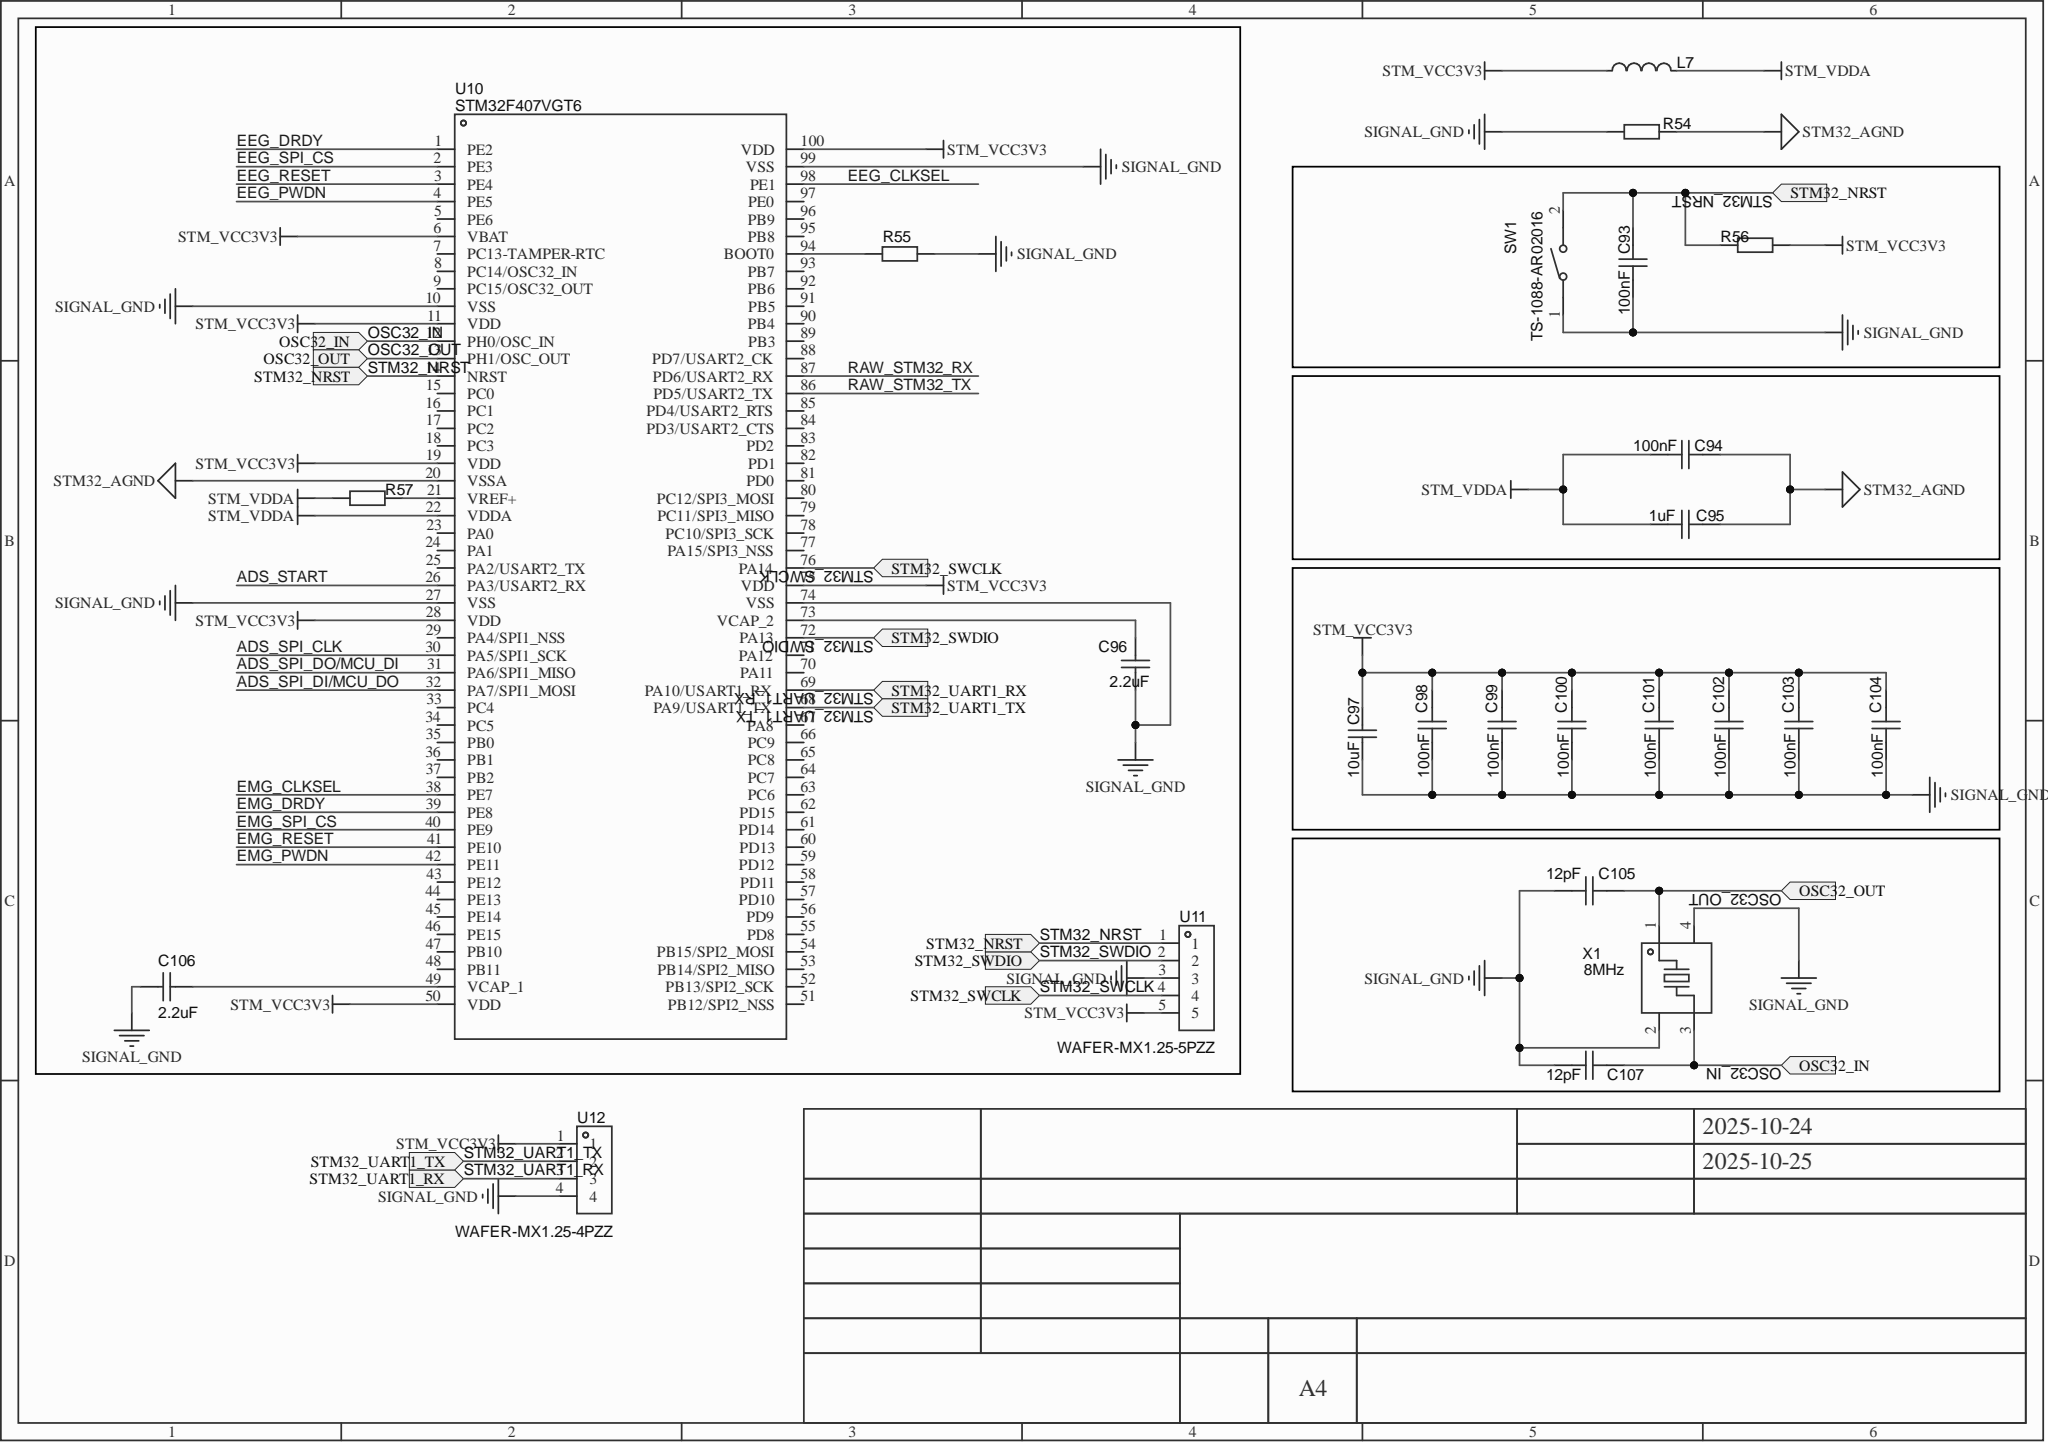Circuit board | Altium Designer | 211 parts | 126 nets | one sheet of the schematic
Parts on this sheet (reference | value | footprint):
C93 | 100nF | C0402
C94 | 100nF | C0402
C95 | 1uF | C0402
C96 | 2.2uF | C0603
C97 | 10uF | C0603
C98 | 100nF | C0402
C99 | 100nF | C0402
C100 | 100nF | C0402
C101 | 100nF | C0402
C102 | 100nF | C0402
C103 | 100nF | C0402
C104 | 100nF | C0402
C105 | 12pF | C0402
C106 | 2.2uF | C0603
C107 | 12pF | C0402
L7 | GZ1608D601TF | L0603
R54 | R0402
R55 | R0402
R56 | R0402
R57 | R0402
SW1 | TS-1088-AR02016 | SW-SMD_L3.9-W3.0-P4.45
U10 | STM32F407VGT6 | LQFP-100_L14.0-W14.0-P0.50-LS16.0-BL
U11 | WAFER-MX1.25-5PZZ | CONN-TH_5P-P1.25_XUNPU_WAFER-MX1.25-5PZZ
U12 | WAFER-MX1.25-4PZZ | CONN-TH_4P-P1.25_WAFER-MX1.25-4PZZ
X1 | 8MHz | CRYSTAL-SMD_4P-L3.2-W2.5-BL
Nets of these parts (net: part-pin ...):
STM_VDDA: C94-2 C95-2 L7-2 R57-1 U10-22
STM_VCC3V3: C97-2 C98-2 C99-2 C100-2 C101-2 C102-2 C103-2 C104-2 L7-1 R56-2 U11-5 U12-1 U10-6 U10-11 U10-19 U10-28 U10-50 U10-75 U10-100
STM32_UART1_TX: U12-2 U10-68
STM32_UART1_RX: U12-3 U10-69
STM32_SWDIO: U11-2 U10-72
STM32_SWCLK: U11-4 U10-76
STM32_NRST: C93-2 R56-1 SW1-2 U11-1 U10-14
STM32_AGND: C94-1 C95-1 R54-2 U10-20
SIGNAL_GND: C93-1 C96-1 C97-1 C98-1 C99-1 C100-1 C101-1 C102-1 C103-1 C104-1 C105-1 C106-2 C107-1 R54-1 R55-2 SW1-1 U11-3 U12-4 X1-2 X1-4 U10-10 U10-27 U10-74 U10-99
RAW_STM32_TX: U10-86
RAW_STM32_RX: U10-87
OSC32_OUT: C105-2 X1-1 U10-13
OSC32_IN: C107-2 X1-3 U10-12
NetR57_2: R57-2 U10-21
NetR55_1: R55-1 U10-94
NetC106_1: C106-1 U10-49
NetC96_2: C96-2 U10-73
EMG_SPI_CS: U10-40
EMG_RESET: U10-41
EMG_PWDN: U10-42
EMG_DRDY: U10-39
EMG_CLKSEL: U10-38
EEG_SPI_CS: U10-2
EEG_RESET: U10-3
EEG_PWDN: U10-4
EEG_DRDY: U10-1
EEG_CLKSEL: U10-98
ADS_START: U10-26
ADS_SPI_DO/MCU_DI: U10-31
ADS_SPI_DI/MCU_DO: U10-32
ADS_SPI_CLK: U10-30